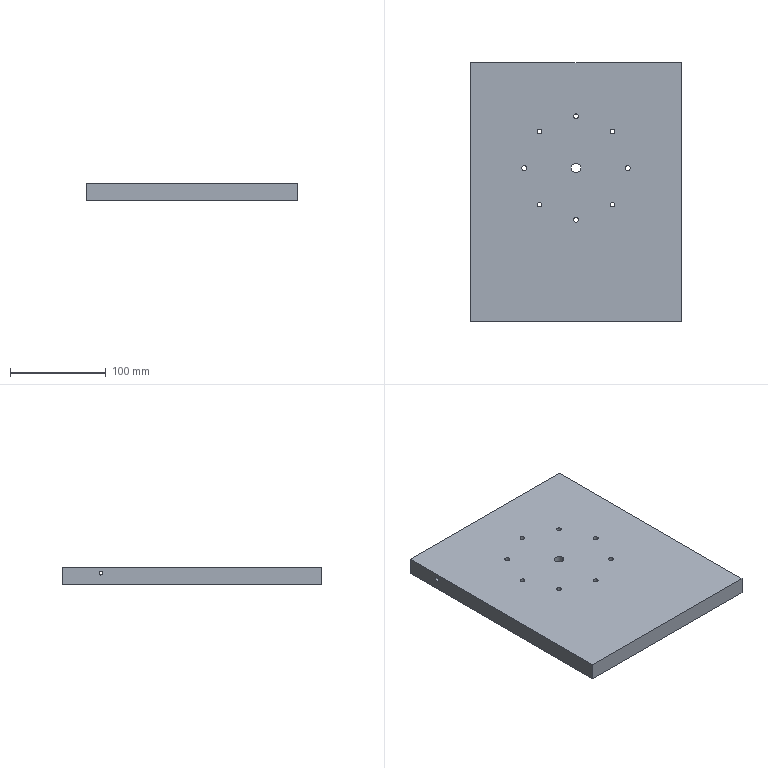Part | SolidWorks | features ICE 5, Extrusion 1 | 1 solid | 26 faces | box 220 x 270 x 18 mm | volume 1062194 mm3 | cylinder 20 | plane 6 | commonest cylinder face diameters 5 x16 4 x2 10 x2
STEP:
#1=CARTESIAN_POINT('',(-110.,100.,14.));
#2=VERTEX_POINT('',#1);
#3=CARTESIAN_POINT('',(-110.,100.,10.));
#4=VERTEX_POINT('',#3);
#5=CARTESIAN_POINT('',(-110.,100.,12.));
#6=DIRECTION('',(1.,0.,0.));
#7=DIRECTION('',(0.,0.,-1.));
#8=AXIS2_PLACEMENT_3D('',#5,#6,#7);
#9=CIRCLE('',#8,2.);
#10=EDGE_CURVE('',#2,#4,#9,.T.);
#11=ORIENTED_EDGE('',*,*,#10,.F.);
#12=CARTESIAN_POINT('',(110.,100.,14.));
#13=VERTEX_POINT('',#12);
#14=CARTESIAN_POINT('',(-110.,100.,14.));
#15=DIRECTION('',(1.,0.,0.));
#16=VECTOR('',#15,1000.);
#17=LINE('',#14,#16);
#18=EDGE_CURVE('',#2,#13,#17,.T.);
#19=ORIENTED_EDGE('',*,*,#18,.T.);
#20=CARTESIAN_POINT('',(110.,100.,10.));
#21=VERTEX_POINT('',#20);
#22=CARTESIAN_POINT('',(110.,100.,12.));
#23=DIRECTION('',(1.,0.,0.));
#24=DIRECTION('',(0.,0.,-1.));
#25=AXIS2_PLACEMENT_3D('',#22,#23,#24);
#26=CIRCLE('',#25,2.);
#27=EDGE_CURVE('',#13,#21,#26,.T.);
#28=ORIENTED_EDGE('',*,*,#27,.T.);
#29=CARTESIAN_POINT('',(-110.,100.,10.));
#30=DIRECTION('',(1.,0.,0.));
#31=VECTOR('',#30,1000.);
#32=LINE('',#29,#31);
#33=EDGE_CURVE('',#4,#21,#32,.T.);
#34=ORIENTED_EDGE('',*,*,#33,.F.);
#35=EDGE_LOOP('',(#11,#19,#28,#34));
#36=FACE_OUTER_BOUND('',#35,.T.);
#37=CARTESIAN_POINT('',(-110.,100.,12.));
#38=DIRECTION('',(1.,0.,0.));
#39=DIRECTION('',(0.,0.,-1.));
#40=AXIS2_PLACEMENT_3D('',#37,#38,#39);
#41=CYLINDRICAL_SURFACE('',#40,2.);
#42=ADVANCED_FACE('',(#36),#41,.F.);
#43=CARTESIAN_POINT('',(-35.684,68.184,18.));
#44=VERTEX_POINT('',#43);
#45=CARTESIAN_POINT('',(-40.684,68.184,18.));
#46=VERTEX_POINT('',#45);
#47=CARTESIAN_POINT('',(-38.184,68.184,18.));
#48=DIRECTION('',(0.,0.,-1.));
#49=DIRECTION('',(-1.,0.,0.));
#50=AXIS2_PLACEMENT_3D('',#47,#48,#49);
#51=CIRCLE('',#50,2.5);
#52=EDGE_CURVE('',#44,#46,#51,.T.);
#53=ORIENTED_EDGE('',*,*,#52,.F.);
#54=CARTESIAN_POINT('',(-35.684,68.184,0.));
#55=VERTEX_POINT('',#54);
#56=CARTESIAN_POINT('',(-35.684,68.184,18.));
#57=DIRECTION('',(0.,0.,-1.));
#58=VECTOR('',#57,1000.);
#59=LINE('',#56,#58);
#60=EDGE_CURVE('',#44,#55,#59,.T.);
#61=ORIENTED_EDGE('',*,*,#60,.T.);
#62=CARTESIAN_POINT('',(-40.684,68.184,0.));
#63=VERTEX_POINT('',#62);
#64=CARTESIAN_POINT('',(-38.184,68.184,0.));
#65=DIRECTION('',(0.,0.,-1.));
#66=DIRECTION('',(-1.,0.,0.));
#67=AXIS2_PLACEMENT_3D('',#64,#65,#66);
#68=CIRCLE('',#67,2.5);
#69=EDGE_CURVE('',#55,#63,#68,.T.);
#70=ORIENTED_EDGE('',*,*,#69,.T.);
#71=CARTESIAN_POINT('',(-40.684,68.184,18.));
#72=DIRECTION('',(0.,0.,-1.));
#73=VECTOR('',#72,1000.);
#74=LINE('',#71,#73);
#75=EDGE_CURVE('',#46,#63,#74,.T.);
#76=ORIENTED_EDGE('',*,*,#75,.F.);
#77=EDGE_LOOP('',(#53,#61,#70,#76));
#78=FACE_OUTER_BOUND('',#77,.T.);
#79=CARTESIAN_POINT('',(-38.184,68.184,18.));
#80=DIRECTION('',(0.,0.,-1.));
#81=DIRECTION('',(-1.,0.,0.));
#82=AXIS2_PLACEMENT_3D('',#79,#80,#81);
#83=CYLINDRICAL_SURFACE('',#82,2.5);
#84=ADVANCED_FACE('',(#78),#83,.F.);
#85=CARTESIAN_POINT('',(-51.5,30.,18.));
#86=VERTEX_POINT('',#85);
#87=CARTESIAN_POINT('',(-56.5,30.,18.));
#88=VERTEX_POINT('',#87);
#89=CARTESIAN_POINT('',(-54.,30.,18.));
#90=DIRECTION('',(0.,0.,-1.));
#91=DIRECTION('',(-1.,0.,0.));
#92=AXIS2_PLACEMENT_3D('',#89,#90,#91);
#93=CIRCLE('',#92,2.5);
#94=EDGE_CURVE('',#86,#88,#93,.T.);
#95=ORIENTED_EDGE('',*,*,#94,.F.);
#96=CARTESIAN_POINT('',(-51.5,30.,0.));
#97=VERTEX_POINT('',#96);
#98=CARTESIAN_POINT('',(-51.5,30.,18.));
#99=DIRECTION('',(0.,0.,-1.));
#100=VECTOR('',#99,1000.);
#101=LINE('',#98,#100);
#102=EDGE_CURVE('',#86,#97,#101,.T.);
#103=ORIENTED_EDGE('',*,*,#102,.T.);
#104=CARTESIAN_POINT('',(-56.5,30.,0.));
#105=VERTEX_POINT('',#104);
#106=CARTESIAN_POINT('',(-54.,30.,0.));
#107=DIRECTION('',(0.,0.,-1.));
#108=DIRECTION('',(-1.,0.,0.));
#109=AXIS2_PLACEMENT_3D('',#106,#107,#108);
#110=CIRCLE('',#109,2.5);
#111=EDGE_CURVE('',#97,#105,#110,.T.);
#112=ORIENTED_EDGE('',*,*,#111,.T.);
#113=CARTESIAN_POINT('',(-56.5,30.,18.));
#114=DIRECTION('',(0.,0.,-1.));
#115=VECTOR('',#114,1000.);
#116=LINE('',#113,#115);
#117=EDGE_CURVE('',#88,#105,#116,.T.);
#118=ORIENTED_EDGE('',*,*,#117,.F.);
#119=EDGE_LOOP('',(#95,#103,#112,#118));
#120=FACE_OUTER_BOUND('',#119,.T.);
#121=CARTESIAN_POINT('',(-54.,30.,18.));
#122=DIRECTION('',(0.,0.,-1.));
#123=DIRECTION('',(-1.,0.,0.));
#124=AXIS2_PLACEMENT_3D('',#121,#122,#123);
#125=CYLINDRICAL_SURFACE('',#124,2.5);
#126=ADVANCED_FACE('',(#120),#125,.F.);
#127=CARTESIAN_POINT('',(-35.684,-8.184,18.));
#128=VERTEX_POINT('',#127);
#129=CARTESIAN_POINT('',(-40.684,-8.184,18.));
#130=VERTEX_POINT('',#129);
#131=CARTESIAN_POINT('',(-38.184,-8.184,18.));
#132=DIRECTION('',(0.,0.,-1.));
#133=DIRECTION('',(-1.,0.,0.));
#134=AXIS2_PLACEMENT_3D('',#131,#132,#133);
#135=CIRCLE('',#134,2.5);
#136=EDGE_CURVE('',#128,#130,#135,.T.);
#137=ORIENTED_EDGE('',*,*,#136,.F.);
#138=CARTESIAN_POINT('',(-35.684,-8.184,0.));
#139=VERTEX_POINT('',#138);
#140=CARTESIAN_POINT('',(-35.684,-8.184,18.));
#141=DIRECTION('',(0.,0.,-1.));
#142=VECTOR('',#141,1000.);
#143=LINE('',#140,#142);
#144=EDGE_CURVE('',#128,#139,#143,.T.);
#145=ORIENTED_EDGE('',*,*,#144,.T.);
#146=CARTESIAN_POINT('',(-40.684,-8.184,0.));
#147=VERTEX_POINT('',#146);
#148=CARTESIAN_POINT('',(-38.184,-8.184,0.));
#149=DIRECTION('',(0.,0.,-1.));
#150=DIRECTION('',(-1.,0.,0.));
#151=AXIS2_PLACEMENT_3D('',#148,#149,#150);
#152=CIRCLE('',#151,2.5);
#153=EDGE_CURVE('',#139,#147,#152,.T.);
#154=ORIENTED_EDGE('',*,*,#153,.T.);
#155=CARTESIAN_POINT('',(-40.684,-8.184,18.));
#156=DIRECTION('',(0.,0.,-1.));
#157=VECTOR('',#156,1000.);
#158=LINE('',#155,#157);
#159=EDGE_CURVE('',#130,#147,#158,.T.);
#160=ORIENTED_EDGE('',*,*,#159,.F.);
#161=EDGE_LOOP('',(#137,#145,#154,#160));
#162=FACE_OUTER_BOUND('',#161,.T.);
#163=CARTESIAN_POINT('',(-38.184,-8.184,18.));
#164=DIRECTION('',(0.,0.,-1.));
#165=DIRECTION('',(-1.,0.,0.));
#166=AXIS2_PLACEMENT_3D('',#163,#164,#165);
#167=CYLINDRICAL_SURFACE('',#166,2.5);
#168=ADVANCED_FACE('',(#162),#167,.F.);
#169=CARTESIAN_POINT('',(2.5,-24.,18.));
#170=VERTEX_POINT('',#169);
#171=CARTESIAN_POINT('',(-2.5,-24.,18.));
#172=VERTEX_POINT('',#171);
#173=CARTESIAN_POINT('',(0.,-24.,18.));
#174=DIRECTION('',(0.,0.,-1.));
#175=DIRECTION('',(-1.,0.,0.));
#176=AXIS2_PLACEMENT_3D('',#173,#174,#175);
#177=CIRCLE('',#176,2.5);
#178=EDGE_CURVE('',#170,#172,#177,.T.);
#179=ORIENTED_EDGE('',*,*,#178,.F.);
#180=CARTESIAN_POINT('',(2.5,-24.,0.));
#181=VERTEX_POINT('',#180);
#182=CARTESIAN_POINT('',(2.5,-24.,18.));
#183=DIRECTION('',(0.,0.,-1.));
#184=VECTOR('',#183,1000.);
#185=LINE('',#182,#184);
#186=EDGE_CURVE('',#170,#181,#185,.T.);
#187=ORIENTED_EDGE('',*,*,#186,.T.);
#188=CARTESIAN_POINT('',(-2.5,-24.,0.));
#189=VERTEX_POINT('',#188);
#190=CARTESIAN_POINT('',(0.,-24.,0.));
#191=DIRECTION('',(0.,0.,-1.));
#192=DIRECTION('',(-1.,0.,0.));
#193=AXIS2_PLACEMENT_3D('',#190,#191,#192);
#194=CIRCLE('',#193,2.5);
#195=EDGE_CURVE('',#181,#189,#194,.T.);
#196=ORIENTED_EDGE('',*,*,#195,.T.);
#197=CARTESIAN_POINT('',(-2.5,-24.,18.));
#198=DIRECTION('',(0.,0.,-1.));
#199=VECTOR('',#198,1000.);
#200=LINE('',#197,#199);
#201=EDGE_CURVE('',#172,#189,#200,.T.);
#202=ORIENTED_EDGE('',*,*,#201,.F.);
#203=EDGE_LOOP('',(#179,#187,#196,#202));
#204=FACE_OUTER_BOUND('',#203,.T.);
#205=CARTESIAN_POINT('',(0.,-24.,18.));
#206=DIRECTION('',(0.,0.,-1.));
#207=DIRECTION('',(-1.,0.,0.));
#208=AXIS2_PLACEMENT_3D('',#205,#206,#207);
#209=CYLINDRICAL_SURFACE('',#208,2.5);
#210=ADVANCED_FACE('',(#204),#209,.F.);
#211=CARTESIAN_POINT('',(40.684,-8.184,18.));
#212=VERTEX_POINT('',#211);
#213=CARTESIAN_POINT('',(35.684,-8.184,18.));
#214=VERTEX_POINT('',#213);
#215=CARTESIAN_POINT('',(38.184,-8.184,18.));
#216=DIRECTION('',(0.,0.,-1.));
#217=DIRECTION('',(-1.,0.,0.));
#218=AXIS2_PLACEMENT_3D('',#215,#216,#217);
#219=CIRCLE('',#218,2.5);
#220=EDGE_CURVE('',#212,#214,#219,.T.);
#221=ORIENTED_EDGE('',*,*,#220,.F.);
#222=CARTESIAN_POINT('',(40.684,-8.184,0.));
#223=VERTEX_POINT('',#222);
#224=CARTESIAN_POINT('',(40.684,-8.184,18.));
#225=DIRECTION('',(0.,0.,-1.));
#226=VECTOR('',#225,1000.);
#227=LINE('',#224,#226);
#228=EDGE_CURVE('',#212,#223,#227,.T.);
#229=ORIENTED_EDGE('',*,*,#228,.T.);
#230=CARTESIAN_POINT('',(35.684,-8.184,0.));
#231=VERTEX_POINT('',#230);
#232=CARTESIAN_POINT('',(38.184,-8.184,0.));
#233=DIRECTION('',(0.,0.,-1.));
#234=DIRECTION('',(-1.,0.,0.));
#235=AXIS2_PLACEMENT_3D('',#232,#233,#234);
#236=CIRCLE('',#235,2.5);
#237=EDGE_CURVE('',#223,#231,#236,.T.);
#238=ORIENTED_EDGE('',*,*,#237,.T.);
#239=CARTESIAN_POINT('',(35.684,-8.184,18.));
#240=DIRECTION('',(0.,0.,-1.));
#241=VECTOR('',#240,1000.);
#242=LINE('',#239,#241);
#243=EDGE_CURVE('',#214,#231,#242,.T.);
#244=ORIENTED_EDGE('',*,*,#243,.F.);
#245=EDGE_LOOP('',(#221,#229,#238,#244));
#246=FACE_OUTER_BOUND('',#245,.T.);
#247=CARTESIAN_POINT('',(38.184,-8.184,18.));
#248=DIRECTION('',(0.,0.,-1.));
#249=DIRECTION('',(-1.,0.,0.));
#250=AXIS2_PLACEMENT_3D('',#247,#248,#249);
#251=CYLINDRICAL_SURFACE('',#250,2.5);
#252=ADVANCED_FACE('',(#246),#251,.F.);
#253=CARTESIAN_POINT('',(56.5,30.,18.));
#254=VERTEX_POINT('',#253);
#255=CARTESIAN_POINT('',(51.5,30.,18.));
#256=VERTEX_POINT('',#255);
#257=CARTESIAN_POINT('',(54.,30.,18.));
#258=DIRECTION('',(0.,0.,-1.));
#259=DIRECTION('',(-1.,0.,0.));
#260=AXIS2_PLACEMENT_3D('',#257,#258,#259);
#261=CIRCLE('',#260,2.5);
#262=EDGE_CURVE('',#254,#256,#261,.T.);
#263=ORIENTED_EDGE('',*,*,#262,.F.);
#264=CARTESIAN_POINT('',(56.5,30.,0.));
#265=VERTEX_POINT('',#264);
#266=CARTESIAN_POINT('',(56.5,30.,18.));
#267=DIRECTION('',(0.,0.,-1.));
#268=VECTOR('',#267,1000.);
#269=LINE('',#266,#268);
#270=EDGE_CURVE('',#254,#265,#269,.T.);
#271=ORIENTED_EDGE('',*,*,#270,.T.);
#272=CARTESIAN_POINT('',(51.5,30.,0.));
#273=VERTEX_POINT('',#272);
#274=CARTESIAN_POINT('',(54.,30.,0.));
#275=DIRECTION('',(0.,0.,-1.));
#276=DIRECTION('',(-1.,0.,0.));
#277=AXIS2_PLACEMENT_3D('',#274,#275,#276);
#278=CIRCLE('',#277,2.5);
#279=EDGE_CURVE('',#265,#273,#278,.T.);
#280=ORIENTED_EDGE('',*,*,#279,.T.);
#281=CARTESIAN_POINT('',(51.5,30.,18.));
#282=DIRECTION('',(0.,0.,-1.));
#283=VECTOR('',#282,1000.);
#284=LINE('',#281,#283);
#285=EDGE_CURVE('',#256,#273,#284,.T.);
#286=ORIENTED_EDGE('',*,*,#285,.F.);
#287=EDGE_LOOP('',(#263,#271,#280,#286));
#288=FACE_OUTER_BOUND('',#287,.T.);
#289=CARTESIAN_POINT('',(54.,30.,18.));
#290=DIRECTION('',(0.,0.,-1.));
#291=DIRECTION('',(-1.,0.,0.));
#292=AXIS2_PLACEMENT_3D('',#289,#290,#291);
#293=CYLINDRICAL_SURFACE('',#292,2.5);
#294=ADVANCED_FACE('',(#288),#293,.F.);
#295=CARTESIAN_POINT('',(2.5,84.,18.));
#296=VERTEX_POINT('',#295);
#297=CARTESIAN_POINT('',(-2.5,84.,18.));
#298=VERTEX_POINT('',#297);
#299=CARTESIAN_POINT('',(0.,84.,18.));
#300=DIRECTION('',(0.,0.,-1.));
#301=DIRECTION('',(-1.,0.,0.));
#302=AXIS2_PLACEMENT_3D('',#299,#300,#301);
#303=CIRCLE('',#302,2.5);
#304=EDGE_CURVE('',#296,#298,#303,.T.);
#305=ORIENTED_EDGE('',*,*,#304,.F.);
#306=CARTESIAN_POINT('',(2.5,84.,0.));
#307=VERTEX_POINT('',#306);
#308=CARTESIAN_POINT('',(2.5,84.,18.));
#309=DIRECTION('',(0.,0.,-1.));
#310=VECTOR('',#309,1000.);
#311=LINE('',#308,#310);
#312=EDGE_CURVE('',#296,#307,#311,.T.);
#313=ORIENTED_EDGE('',*,*,#312,.T.);
#314=CARTESIAN_POINT('',(-2.5,84.,0.));
#315=VERTEX_POINT('',#314);
#316=CARTESIAN_POINT('',(0.,84.,0.));
#317=DIRECTION('',(0.,0.,-1.));
#318=DIRECTION('',(-1.,0.,0.));
#319=AXIS2_PLACEMENT_3D('',#316,#317,#318);
#320=CIRCLE('',#319,2.5);
#321=EDGE_CURVE('',#307,#315,#320,.T.);
#322=ORIENTED_EDGE('',*,*,#321,.T.);
#323=CARTESIAN_POINT('',(-2.5,84.,18.));
#324=DIRECTION('',(0.,0.,-1.));
#325=VECTOR('',#324,1000.);
#326=LINE('',#323,#325);
#327=EDGE_CURVE('',#298,#315,#326,.T.);
#328=ORIENTED_EDGE('',*,*,#327,.F.);
#329=EDGE_LOOP('',(#305,#313,#322,#328));
#330=FACE_OUTER_BOUND('',#329,.T.);
#331=CARTESIAN_POINT('',(0.,84.,18.));
#332=DIRECTION('',(0.,0.,-1.));
#333=DIRECTION('',(-1.,0.,0.));
#334=AXIS2_PLACEMENT_3D('',#331,#332,#333);
#335=CYLINDRICAL_SURFACE('',#334,2.5);
#336=ADVANCED_FACE('',(#330),#335,.F.);
#337=CARTESIAN_POINT('',(40.684,68.184,18.));
#338=VERTEX_POINT('',#337);
#339=CARTESIAN_POINT('',(35.684,68.184,18.));
#340=VERTEX_POINT('',#339);
#341=CARTESIAN_POINT('',(38.184,68.184,18.));
#342=DIRECTION('',(0.,0.,-1.));
#343=DIRECTION('',(-1.,0.,0.));
#344=AXIS2_PLACEMENT_3D('',#341,#342,#343);
#345=CIRCLE('',#344,2.5);
#346=EDGE_CURVE('',#338,#340,#345,.T.);
#347=ORIENTED_EDGE('',*,*,#346,.F.);
#348=CARTESIAN_POINT('',(40.684,68.184,0.));
#349=VERTEX_POINT('',#348);
#350=CARTESIAN_POINT('',(40.684,68.184,18.));
#351=DIRECTION('',(0.,0.,-1.));
#352=VECTOR('',#351,1000.);
#353=LINE('',#350,#352);
#354=EDGE_CURVE('',#338,#349,#353,.T.);
#355=ORIENTED_EDGE('',*,*,#354,.T.);
#356=CARTESIAN_POINT('',(35.684,68.184,0.));
#357=VERTEX_POINT('',#356);
#358=CARTESIAN_POINT('',(38.184,68.184,0.));
#359=DIRECTION('',(0.,0.,-1.));
#360=DIRECTION('',(-1.,0.,0.));
#361=AXIS2_PLACEMENT_3D('',#358,#359,#360);
#362=CIRCLE('',#361,2.5);
#363=EDGE_CURVE('',#349,#357,#362,.T.);
#364=ORIENTED_EDGE('',*,*,#363,.T.);
#365=CARTESIAN_POINT('',(35.684,68.184,18.));
#366=DIRECTION('',(0.,0.,-1.));
#367=VECTOR('',#366,1000.);
#368=LINE('',#365,#367);
#369=EDGE_CURVE('',#340,#357,#368,.T.);
#370=ORIENTED_EDGE('',*,*,#369,.F.);
#371=EDGE_LOOP('',(#347,#355,#364,#370));
#372=FACE_OUTER_BOUND('',#371,.T.);
#373=CARTESIAN_POINT('',(38.184,68.184,18.));
#374=DIRECTION('',(0.,0.,-1.));
#375=DIRECTION('',(-1.,0.,0.));
#376=AXIS2_PLACEMENT_3D('',#373,#374,#375);
#377=CYLINDRICAL_SURFACE('',#376,2.5);
#378=ADVANCED_FACE('',(#372),#377,.F.);
#379=CARTESIAN_POINT('',(-5.,30.,18.));
#380=VERTEX_POINT('',#379);
#381=CARTESIAN_POINT('',(5.,30.,18.));
#382=VERTEX_POINT('',#381);
#383=CARTESIAN_POINT('',(0.,30.,18.));
#384=DIRECTION('',(0.,0.,1.));
#385=DIRECTION('',(1.,0.,0.));
#386=AXIS2_PLACEMENT_3D('',#383,#384,#385);
#387=CIRCLE('',#386,5.);
#388=EDGE_CURVE('',#380,#382,#387,.T.);
#389=ORIENTED_EDGE('',*,*,#388,.T.);
#390=CARTESIAN_POINT('',(5.,30.,0.));
#391=VERTEX_POINT('',#390);
#392=CARTESIAN_POINT('',(5.,30.,18.));
#393=DIRECTION('',(0.,0.,-1.));
#394=VECTOR('',#393,1000.);
#395=LINE('',#392,#394);
#396=EDGE_CURVE('',#382,#391,#395,.T.);
#397=ORIENTED_EDGE('',*,*,#396,.T.);
#398=CARTESIAN_POINT('',(-5.,30.,0.));
#399=VERTEX_POINT('',#398);
#400=CARTESIAN_POINT('',(0.,30.,0.));
#401=DIRECTION('',(0.,0.,1.));
#402=DIRECTION('',(1.,0.,0.));
#403=AXIS2_PLACEMENT_3D('',#400,#401,#402);
#404=CIRCLE('',#403,5.);
#405=EDGE_CURVE('',#399,#391,#404,.T.);
#406=ORIENTED_EDGE('',*,*,#405,.F.);
#407=CARTESIAN_POINT('',(-5.,30.,18.));
#408=DIRECTION('',(0.,0.,-1.));
#409=VECTOR('',#408,1000.);
#410=LINE('',#407,#409);
#411=EDGE_CURVE('',#380,#399,#410,.T.);
#412=ORIENTED_EDGE('',*,*,#411,.F.);
#413=EDGE_LOOP('',(#389,#397,#406,#412));
#414=FACE_OUTER_BOUND('',#413,.T.);
#415=CARTESIAN_POINT('',(0.,30.,18.));
#416=DIRECTION('',(0.,0.,-1.));
#417=DIRECTION('',(-1.,0.,0.));
#418=AXIS2_PLACEMENT_3D('',#415,#416,#417);
#419=CYLINDRICAL_SURFACE('',#418,5.);
#420=ADVANCED_FACE('',(#414),#419,.F.);
#421=CARTESIAN_POINT('',(110.,100.,12.));
#422=DIRECTION('',(1.,0.,0.));
#423=DIRECTION('',(0.,0.,-1.));
#424=AXIS2_PLACEMENT_3D('',#421,#422,#423);
#425=CIRCLE('',#424,2.);
#426=EDGE_CURVE('',#21,#13,#425,.T.);
#427=ORIENTED_EDGE('',*,*,#426,.F.);
#428=ORIENTED_EDGE('',*,*,#27,.F.);
#429=EDGE_LOOP('',(#427,#428));
#430=FACE_BOUND('',#429,.T.);
#431=CARTESIAN_POINT('',(110.,-130.,18.));
#432=VERTEX_POINT('',#431);
#433=CARTESIAN_POINT('',(110.,140.,18.));
#434=VERTEX_POINT('',#433);
#435=CARTESIAN_POINT('',(110.,-140.,18.));
#436=DIRECTION('',(0.,1.,0.));
#437=VECTOR('',#436,1000.);
#438=LINE('',#435,#437);
#439=EDGE_CURVE('',#432,#434,#438,.T.);
#440=ORIENTED_EDGE('',*,*,#439,.F.);
#441=CARTESIAN_POINT('',(110.,-130.,0.));
#442=VERTEX_POINT('',#441);
#443=CARTESIAN_POINT('',(110.,-130.,0.));
#444=DIRECTION('',(0.,0.,1.));
#445=VECTOR('',#444,1000.);
#446=LINE('',#443,#445);
#447=EDGE_CURVE('',#442,#432,#446,.T.);
#448=ORIENTED_EDGE('',*,*,#447,.F.);
#449=CARTESIAN_POINT('',(110.,140.,0.));
#450=VERTEX_POINT('',#449);
#451=CARTESIAN_POINT('',(110.,-140.,0.));
#452=DIRECTION('',(0.,1.,0.));
#453=VECTOR('',#452,1000.);
#454=LINE('',#451,#453);
#455=EDGE_CURVE('',#442,#450,#454,.T.);
#456=ORIENTED_EDGE('',*,*,#455,.T.);
#457=CARTESIAN_POINT('',(110.,140.,18.));
#458=DIRECTION('',(0.,0.,-1.));
#459=VECTOR('',#458,1000.);
#460=LINE('',#457,#459);
#461=EDGE_CURVE('',#434,#450,#460,.T.);
#462=ORIENTED_EDGE('',*,*,#461,.F.);
#463=EDGE_LOOP('',(#440,#448,#456,#462));
#464=FACE_OUTER_BOUND('',#463,.T.);
#465=CARTESIAN_POINT('',(110.,-140.,18.));
#466=DIRECTION('',(-1.,0.,0.));
#467=DIRECTION('',(0.,0.,1.));
#468=AXIS2_PLACEMENT_3D('',#465,#466,#467);
#469=PLANE('',#468);
#470=ADVANCED_FACE('',(#430,#464),#469,.F.);
#471=CARTESIAN_POINT('',(-110.,100.,12.));
#472=DIRECTION('',(1.,0.,0.));
#473=DIRECTION('',(0.,0.,-1.));
#474=AXIS2_PLACEMENT_3D('',#471,#472,#473);
#475=CIRCLE('',#474,2.);
#476=EDGE_CURVE('',#4,#2,#475,.T.);
#477=ORIENTED_EDGE('',*,*,#476,.T.);
#478=ORIENTED_EDGE('',*,*,#10,.T.);
#479=EDGE_LOOP('',(#477,#478));
#480=FACE_BOUND('',#479,.T.);
#481=CARTESIAN_POINT('',(-110.,140.,0.));
#482=VERTEX_POINT('',#481);
#483=CARTESIAN_POINT('',(-110.,-130.,0.));
#484=VERTEX_POINT('',#483);
#485=CARTESIAN_POINT('',(-110.,-140.,0.));
#486=DIRECTION('',(0.,-1.,0.));
#487=VECTOR('',#486,1000.);
#488=LINE('',#485,#487);
#489=EDGE_CURVE('',#482,#484,#488,.T.);
#490=ORIENTED_EDGE('',*,*,#489,.T.);
#491=CARTESIAN_POINT('',(-110.,-130.,18.));
#492=VERTEX_POINT('',#491);
#493=CARTESIAN_POINT('',(-110.,-130.,0.));
#494=DIRECTION('',(0.,0.,1.));
#495=VECTOR('',#494,1000.);
#496=LINE('',#493,#495);
#497=EDGE_CURVE('',#484,#492,#496,.T.);
#498=ORIENTED_EDGE('',*,*,#497,.T.);
#499=CARTESIAN_POINT('',(-110.,140.,18.));
#500=VERTEX_POINT('',#499);
#501=CARTESIAN_POINT('',(-110.,-140.,18.));
#502=DIRECTION('',(0.,-1.,0.));
#503=VECTOR('',#502,1000.);
#504=LINE('',#501,#503);
#505=EDGE_CURVE('',#500,#492,#504,.T.);
#506=ORIENTED_EDGE('',*,*,#505,.F.);
#507=CARTESIAN_POINT('',(-110.,140.,18.));
#508=DIRECTION('',(0.,0.,-1.));
#509=VECTOR('',#508,1000.);
#510=LINE('',#507,#509);
#511=EDGE_CURVE('',#500,#482,#510,.T.);
#512=ORIENTED_EDGE('',*,*,#511,.T.);
#513=EDGE_LOOP('',(#490,#498,#506,#512));
#514=FACE_OUTER_BOUND('',#513,.T.);
#515=CARTESIAN_POINT('',(-110.,-140.,18.));
#516=DIRECTION('',(1.,0.,0.));
#517=DIRECTION('',(0.,0.,-1.));
#518=AXIS2_PLACEMENT_3D('',#515,#516,#517);
#519=PLANE('',#518);
#520=ADVANCED_FACE('',(#480,#514),#519,.F.);
#521=CARTESIAN_POINT('',(-38.184,68.184,18.));
#522=DIRECTION('',(0.,0.,-1.));
#523=DIRECTION('',(-1.,0.,0.));
#524=AXIS2_PLACEMENT_3D('',#521,#522,#523);
#525=CIRCLE('',#524,2.5);
#526=EDGE_CURVE('',#46,#44,#525,.T.);
#527=ORIENTED_EDGE('',*,*,#526,.T.);
#528=ORIENTED_EDGE('',*,*,#52,.T.);
#529=EDGE_LOOP('',(#527,#528));
#530=FACE_BOUND('',#529,.T.);
#531=CARTESIAN_POINT('',(-54.,30.,18.));
#532=DIRECTION('',(0.,0.,-1.));
#533=DIRECTION('',(-1.,0.,0.));
#534=AXIS2_PLACEMENT_3D('',#531,#532,#533);
#535=CIRCLE('',#534,2.5);
#536=EDGE_CURVE('',#88,#86,#535,.T.);
#537=ORIENTED_EDGE('',*,*,#536,.T.);
#538=ORIENTED_EDGE('',*,*,#94,.T.);
#539=EDGE_LOOP('',(#537,#538));
#540=FACE_BOUND('',#539,.T.);
#541=CARTESIAN_POINT('',(-38.184,-8.184,18.));
#542=DIRECTION('',(0.,0.,-1.));
#543=DIRECTION('',(-1.,0.,0.));
#544=AXIS2_PLACEMENT_3D('',#541,#542,#543);
#545=CIRCLE('',#544,2.5);
#546=EDGE_CURVE('',#130,#128,#545,.T.);
#547=ORIENTED_EDGE('',*,*,#546,.T.);
#548=ORIENTED_EDGE('',*,*,#136,.T.);
#549=EDGE_LOOP('',(#547,#548));
#550=FACE_BOUND('',#549,.T.);
#551=CARTESIAN_POINT('',(0.,-24.,18.));
#552=DIRECTION('',(0.,0.,-1.));
#553=DIRECTION('',(-1.,0.,0.));
#554=AXIS2_PLACEMENT_3D('',#551,#552,#553);
#555=CIRCLE('',#554,2.5);
#556=EDGE_CURVE('',#172,#170,#555,.T.);
#557=ORIENTED_EDGE('',*,*,#556,.T.);
#558=ORIENTED_EDGE('',*,*,#178,.T.);
#559=EDGE_LOOP('',(#557,#558));
#560=FACE_BOUND('',#559,.T.);
#561=CARTESIAN_POINT('',(38.184,-8.184,18.));
#562=DIRECTION('',(0.,0.,-1.));
#563=DIRECTION('',(-1.,0.,0.));
#564=AXIS2_PLACEMENT_3D('',#561,#562,#563);
#565=CIRCLE('',#564,2.5);
#566=EDGE_CURVE('',#214,#212,#565,.T.);
#567=ORIENTED_EDGE('',*,*,#566,.T.);
#568=ORIENTED_EDGE('',*,*,#220,.T.);
#569=EDGE_LOOP('',(#567,#568));
#570=FACE_BOUND('',#569,.T.);
#571=CARTESIAN_POINT('',(54.,30.,18.));
#572=DIRECTION('',(0.,0.,-1.));
#573=DIRECTION('',(-1.,0.,0.));
#574=AXIS2_PLACEMENT_3D('',#571,#572,#573);
#575=CIRCLE('',#574,2.5);
#576=EDGE_CURVE('',#256,#254,#575,.T.);
#577=ORIENTED_EDGE('',*,*,#576,.T.);
#578=ORIENTED_EDGE('',*,*,#262,.T.);
#579=EDGE_LOOP('',(#577,#578));
#580=FACE_BOUND('',#579,.T.);
#581=CARTESIAN_POINT('',(0.,84.,18.));
#582=DIRECTION('',(0.,0.,-1.));
#583=DIRECTION('',(-1.,0.,0.));
#584=AXIS2_PLACEMENT_3D('',#581,#582,#583);
#585=CIRCLE('',#584,2.5);
#586=EDGE_CURVE('',#298,#296,#585,.T.);
#587=ORIENTED_EDGE('',*,*,#586,.T.);
#588=ORIENTED_EDGE('',*,*,#304,.T.);
#589=EDGE_LOOP('',(#587,#588));
#590=FACE_BOUND('',#589,.T.);
#591=CARTESIAN_POINT('',(38.184,68.184,18.));
#592=DIRECTION('',(0.,0.,-1.));
#593=DIRECTION('',(-1.,0.,0.));
#594=AXIS2_PLACEMENT_3D('',#591,#592,#593);
#595=CIRCLE('',#594,2.5);
#596=EDGE_CURVE('',#340,#338,#595,.T.);
#597=ORIENTED_EDGE('',*,*,#596,.T.);
#598=ORIENTED_EDGE('',*,*,#346,.T.);
#599=EDGE_LOOP('',(#597,#598));
#600=FACE_BOUND('',#599,.T.);
#601=ORIENTED_EDGE('',*,*,#388,.F.);
#602=CARTESIAN_POINT('',(0.,30.,18.));
#603=DIRECTION('',(0.,0.,1.));
#604=DIRECTION('',(1.,0.,0.));
#605=AXIS2_PLACEMENT_3D('',#602,#603,#604);
#606=CIRCLE('',#605,5.);
#607=EDGE_CURVE('',#382,#380,#606,.T.);
#608=ORIENTED_EDGE('',*,*,#607,.F.);
#609=EDGE_LOOP('',(#601,#608));
#610=FACE_BOUND('',#609,.T.);
#611=ORIENTED_EDGE('',*,*,#505,.T.);
#612=CARTESIAN_POINT('',(110.,-130.,18.));
#613=DIRECTION('',(-1.,0.,0.));
#614=VECTOR('',#613,1000.);
#615=LINE('',#612,#614);
#616=EDGE_CURVE('',#432,#492,#615,.T.);
#617=ORIENTED_EDGE('',*,*,#616,.F.);
#618=ORIENTED_EDGE('',*,*,#439,.T.);
#619=CARTESIAN_POINT('',(-110.,140.,18.));
#620=DIRECTION('',(-1.,0.,0.));
#621=VECTOR('',#620,1000.);
#622=LINE('',#619,#621);
#623=EDGE_CURVE('',#434,#500,#622,.T.);
#624=ORIENTED_EDGE('',*,*,#623,.T.);
#625=EDGE_LOOP('',(#611,#617,#618,#624));
#626=FACE_OUTER_BOUND('',#625,.T.);
#627=CARTESIAN_POINT('',(0.,0.,18.));
#628=DIRECTION('',(0.,0.,-1.));
#629=DIRECTION('',(-1.,0.,0.));
#630=AXIS2_PLACEMENT_3D('',#627,#628,#629);
#631=PLANE('',#630);
#632=ADVANCED_FACE('',(#530,#540,#550,#560,#570,#580,#590,#600,#610,#626),#631,.F.);
#633=CARTESIAN_POINT('',(-38.184,68.184,0.));
#634=DIRECTION('',(0.,0.,-1.));
#635=DIRECTION('',(-1.,0.,0.));
#636=AXIS2_PLACEMENT_3D('',#633,#634,#635);
#637=CIRCLE('',#636,2.5);
#638=EDGE_CURVE('',#63,#55,#637,.T.);
#639=ORIENTED_EDGE('',*,*,#638,.F.);
#640=ORIENTED_EDGE('',*,*,#69,.F.);
#641=EDGE_LOOP('',(#639,#640));
#642=FACE_BOUND('',#641,.T.);
#643=CARTESIAN_POINT('',(-54.,30.,0.));
#644=DIRECTION('',(0.,0.,-1.));
#645=DIRECTION('',(-1.,0.,0.));
#646=AXIS2_PLACEMENT_3D('',#643,#644,#645);
#647=CIRCLE('',#646,2.5);
#648=EDGE_CURVE('',#105,#97,#647,.T.);
#649=ORIENTED_EDGE('',*,*,#648,.F.);
#650=ORIENTED_EDGE('',*,*,#111,.F.);
#651=EDGE_LOOP('',(#649,#650));
#652=FACE_BOUND('',#651,.T.);
#653=CARTESIAN_POINT('',(-38.184,-8.184,0.));
#654=DIRECTION('',(0.,0.,-1.));
#655=DIRECTION('',(-1.,0.,0.));
#656=AXIS2_PLACEMENT_3D('',#653,#654,#655);
#657=CIRCLE('',#656,2.5);
#658=EDGE_CURVE('',#147,#139,#657,.T.);
#659=ORIENTED_EDGE('',*,*,#658,.F.);
#660=ORIENTED_EDGE('',*,*,#153,.F.);
#661=EDGE_LOOP('',(#659,#660));
#662=FACE_BOUND('',#661,.T.);
#663=CARTESIAN_POINT('',(0.,-24.,0.));
#664=DIRECTION('',(0.,0.,-1.));
#665=DIRECTION('',(-1.,0.,0.));
#666=AXIS2_PLACEMENT_3D('',#663,#664,#665);
#667=CIRCLE('',#666,2.5);
#668=EDGE_CURVE('',#189,#181,#667,.T.);
#669=ORIENTED_EDGE('',*,*,#668,.F.);
#670=ORIENTED_EDGE('',*,*,#195,.F.);
#671=EDGE_LOOP('',(#669,#670));
#672=FACE_BOUND('',#671,.T.);
#673=CARTESIAN_POINT('',(38.184,-8.184,0.));
#674=DIRECTION('',(0.,0.,-1.));
#675=DIRECTION('',(-1.,0.,0.));
#676=AXIS2_PLACEMENT_3D('',#673,#674,#675);
#677=CIRCLE('',#676,2.5);
#678=EDGE_CURVE('',#231,#223,#677,.T.);
#679=ORIENTED_EDGE('',*,*,#678,.F.);
#680=ORIENTED_EDGE('',*,*,#237,.F.);
#681=EDGE_LOOP('',(#679,#680));
#682=FACE_BOUND('',#681,.T.);
#683=CARTESIAN_POINT('',(54.,30.,0.));
#684=DIRECTION('',(0.,0.,-1.));
#685=DIRECTION('',(-1.,0.,0.));
#686=AXIS2_PLACEMENT_3D('',#683,#684,#685);
#687=CIRCLE('',#686,2.5);
#688=EDGE_CURVE('',#273,#265,#687,.T.);
#689=ORIENTED_EDGE('',*,*,#688,.F.);
#690=ORIENTED_EDGE('',*,*,#279,.F.);
#691=EDGE_LOOP('',(#689,#690));
#692=FACE_BOUND('',#691,.T.);
#693=CARTESIAN_POINT('',(0.,84.,0.));
#694=DIRECTION('',(0.,0.,-1.));
#695=DIRECTION('',(-1.,0.,0.));
#696=AXIS2_PLACEMENT_3D('',#693,#694,#695);
#697=CIRCLE('',#696,2.5);
#698=EDGE_CURVE('',#315,#307,#697,.T.);
#699=ORIENTED_EDGE('',*,*,#698,.F.);
#700=ORIENTED_EDGE('',*,*,#321,.F.);
#701=EDGE_LOOP('',(#699,#700));
#702=FACE_BOUND('',#701,.T.);
#703=CARTESIAN_POINT('',(38.184,68.184,0.));
#704=DIRECTION('',(0.,0.,-1.));
#705=DIRECTION('',(-1.,0.,0.));
#706=AXIS2_PLACEMENT_3D('',#703,#704,#705);
#707=CIRCLE('',#706,2.5);
#708=EDGE_CURVE('',#357,#349,#707,.T.);
#709=ORIENTED_EDGE('',*,*,#708,.F.);
#710=ORIENTED_EDGE('',*,*,#363,.F.);
#711=EDGE_LOOP('',(#709,#710));
#712=FACE_BOUND('',#711,.T.);
#713=ORIENTED_EDGE('',*,*,#405,.T.);
#714=CARTESIAN_POINT('',(0.,30.,0.));
#715=DIRECTION('',(0.,0.,1.));
#716=DIRECTION('',(1.,0.,0.));
#717=AXIS2_PLACEMENT_3D('',#714,#715,#716);
#718=CIRCLE('',#717,5.);
#719=EDGE_CURVE('',#391,#399,#718,.T.);
#720=ORIENTED_EDGE('',*,*,#719,.T.);
#721=EDGE_LOOP('',(#713,#720));
#722=FACE_BOUND('',#721,.T.);
#723=ORIENTED_EDGE('',*,*,#455,.F.);
#724=CARTESIAN_POINT('',(110.,-130.,0.));
#725=DIRECTION('',(-1.,0.,0.));
#726=VECTOR('',#725,1000.);
#727=LINE('',#724,#726);
#728=EDGE_CURVE('',#442,#484,#727,.T.);
#729=ORIENTED_EDGE('',*,*,#728,.T.);
#730=ORIENTED_EDGE('',*,*,#489,.F.);
#731=CARTESIAN_POINT('',(-110.,140.,0.));
#732=DIRECTION('',(-1.,0.,0.));
#733=VECTOR('',#732,1000.);
#734=LINE('',#731,#733);
#735=EDGE_CURVE('',#450,#482,#734,.T.);
#736=ORIENTED_EDGE('',*,*,#735,.F.);
#737=EDGE_LOOP('',(#723,#729,#730,#736));
#738=FACE_OUTER_BOUND('',#737,.T.);
#739=CARTESIAN_POINT('',(0.,0.,0.));
#740=DIRECTION('',(0.,0.,-1.));
#741=DIRECTION('',(-1.,0.,0.));
#742=AXIS2_PLACEMENT_3D('',#739,#740,#741);
#743=PLANE('',#742);
#744=ADVANCED_FACE('',(#642,#652,#662,#672,#682,#692,#702,#712,#722,#738),#743,.T.);
#745=ORIENTED_EDGE('',*,*,#735,.T.);
#746=ORIENTED_EDGE('',*,*,#511,.F.);
#747=ORIENTED_EDGE('',*,*,#623,.F.);
#748=ORIENTED_EDGE('',*,*,#461,.T.);
#749=EDGE_LOOP('',(#745,#746,#747,#748));
#750=FACE_OUTER_BOUND('',#749,.T.);
#751=CARTESIAN_POINT('',(-110.,140.,18.));
#752=DIRECTION('',(0.,-1.,0.));
#753=DIRECTION('',(0.,0.,-1.));
#754=AXIS2_PLACEMENT_3D('',#751,#752,#753);
#755=PLANE('',#754);
#756=ADVANCED_FACE('',(#750),#755,.F.);
#757=ORIENTED_EDGE('',*,*,#396,.F.);
#758=ORIENTED_EDGE('',*,*,#607,.T.);
#759=ORIENTED_EDGE('',*,*,#411,.T.);
#760=ORIENTED_EDGE('',*,*,#719,.F.);
#761=EDGE_LOOP('',(#757,#758,#759,#760));
#762=FACE_OUTER_BOUND('',#761,.T.);
#763=CARTESIAN_POINT('',(0.,30.,18.));
#764=DIRECTION('',(0.,0.,-1.));
#765=DIRECTION('',(-1.,0.,0.));
#766=AXIS2_PLACEMENT_3D('',#763,#764,#765);
#767=CYLINDRICAL_SURFACE('',#766,5.);
#768=ADVANCED_FACE('',(#762),#767,.F.);
#769=ORIENTED_EDGE('',*,*,#354,.F.);
#770=ORIENTED_EDGE('',*,*,#596,.F.);
#771=ORIENTED_EDGE('',*,*,#369,.T.);
#772=ORIENTED_EDGE('',*,*,#708,.T.);
#773=EDGE_LOOP('',(#769,#770,#771,#772));
#774=FACE_OUTER_BOUND('',#773,.T.);
#775=CARTESIAN_POINT('',(38.184,68.184,18.));
#776=DIRECTION('',(0.,0.,-1.));
#777=DIRECTION('',(-1.,0.,0.));
#778=AXIS2_PLACEMENT_3D('',#775,#776,#777);
#779=CYLINDRICAL_SURFACE('',#778,2.5);
#780=ADVANCED_FACE('',(#774),#779,.F.);
#781=ORIENTED_EDGE('',*,*,#312,.F.);
#782=ORIENTED_EDGE('',*,*,#586,.F.);
#783=ORIENTED_EDGE('',*,*,#327,.T.);
#784=ORIENTED_EDGE('',*,*,#698,.T.);
#785=EDGE_LOOP('',(#781,#782,#783,#784));
#786=FACE_OUTER_BOUND('',#785,.T.);
#787=CARTESIAN_POINT('',(0.,84.,18.));
#788=DIRECTION('',(0.,0.,-1.));
#789=DIRECTION('',(-1.,0.,0.));
#790=AXIS2_PLACEMENT_3D('',#787,#788,#789);
#791=CYLINDRICAL_SURFACE('',#790,2.5);
#792=ADVANCED_FACE('',(#786),#791,.F.);
#793=ORIENTED_EDGE('',*,*,#270,.F.);
#794=ORIENTED_EDGE('',*,*,#576,.F.);
#795=ORIENTED_EDGE('',*,*,#285,.T.);
#796=ORIENTED_EDGE('',*,*,#688,.T.);
#797=EDGE_LOOP('',(#793,#794,#795,#796));
#798=FACE_OUTER_BOUND('',#797,.T.);
#799=CARTESIAN_POINT('',(54.,30.,18.));
#800=DIRECTION('',(0.,0.,-1.));
#801=DIRECTION('',(-1.,0.,0.));
#802=AXIS2_PLACEMENT_3D('',#799,#800,#801);
#803=CYLINDRICAL_SURFACE('',#802,2.5);
#804=ADVANCED_FACE('',(#798),#803,.F.);
#805=ORIENTED_EDGE('',*,*,#228,.F.);
#806=ORIENTED_EDGE('',*,*,#566,.F.);
#807=ORIENTED_EDGE('',*,*,#243,.T.);
#808=ORIENTED_EDGE('',*,*,#678,.T.);
#809=EDGE_LOOP('',(#805,#806,#807,#808));
#810=FACE_OUTER_BOUND('',#809,.T.);
#811=CARTESIAN_POINT('',(38.184,-8.184,18.));
#812=DIRECTION('',(0.,0.,-1.));
#813=DIRECTION('',(-1.,0.,0.));
#814=AXIS2_PLACEMENT_3D('',#811,#812,#813);
#815=CYLINDRICAL_SURFACE('',#814,2.5);
#816=ADVANCED_FACE('',(#810),#815,.F.);
#817=ORIENTED_EDGE('',*,*,#186,.F.);
#818=ORIENTED_EDGE('',*,*,#556,.F.);
#819=ORIENTED_EDGE('',*,*,#201,.T.);
#820=ORIENTED_EDGE('',*,*,#668,.T.);
#821=EDGE_LOOP('',(#817,#818,#819,#820));
#822=FACE_OUTER_BOUND('',#821,.T.);
#823=CARTESIAN_POINT('',(0.,-24.,18.));
#824=DIRECTION('',(0.,0.,-1.));
#825=DIRECTION('',(-1.,0.,0.));
#826=AXIS2_PLACEMENT_3D('',#823,#824,#825);
#827=CYLINDRICAL_SURFACE('',#826,2.5);
#828=ADVANCED_FACE('',(#822),#827,.F.);
#829=ORIENTED_EDGE('',*,*,#144,.F.);
#830=ORIENTED_EDGE('',*,*,#546,.F.);
#831=ORIENTED_EDGE('',*,*,#159,.T.);
#832=ORIENTED_EDGE('',*,*,#658,.T.);
#833=EDGE_LOOP('',(#829,#830,#831,#832));
#834=FACE_OUTER_BOUND('',#833,.T.);
#835=CARTESIAN_POINT('',(-38.184,-8.184,18.));
#836=DIRECTION('',(0.,0.,-1.));
#837=DIRECTION('',(-1.,0.,0.));
#838=AXIS2_PLACEMENT_3D('',#835,#836,#837);
#839=CYLINDRICAL_SURFACE('',#838,2.5);
#840=ADVANCED_FACE('',(#834),#839,.F.);
#841=ORIENTED_EDGE('',*,*,#102,.F.);
#842=ORIENTED_EDGE('',*,*,#536,.F.);
#843=ORIENTED_EDGE('',*,*,#117,.T.);
#844=ORIENTED_EDGE('',*,*,#648,.T.);
#845=EDGE_LOOP('',(#841,#842,#843,#844));
#846=FACE_OUTER_BOUND('',#845,.T.);
#847=CARTESIAN_POINT('',(-54.,30.,18.));
#848=DIRECTION('',(0.,0.,-1.));
#849=DIRECTION('',(-1.,0.,0.));
#850=AXIS2_PLACEMENT_3D('',#847,#848,#849);
#851=CYLINDRICAL_SURFACE('',#850,2.5);
#852=ADVANCED_FACE('',(#846),#851,.F.);
#853=ORIENTED_EDGE('',*,*,#60,.F.);
#854=ORIENTED_EDGE('',*,*,#526,.F.);
#855=ORIENTED_EDGE('',*,*,#75,.T.);
#856=ORIENTED_EDGE('',*,*,#638,.T.);
#857=EDGE_LOOP('',(#853,#854,#855,#856));
#858=FACE_OUTER_BOUND('',#857,.T.);
#859=CARTESIAN_POINT('',(-38.184,68.184,18.));
#860=DIRECTION('',(0.,0.,-1.));
#861=DIRECTION('',(-1.,0.,0.));
#862=AXIS2_PLACEMENT_3D('',#859,#860,#861);
#863=CYLINDRICAL_SURFACE('',#862,2.5);
#864=ADVANCED_FACE('',(#858),#863,.F.);
#865=ORIENTED_EDGE('',*,*,#497,.F.);
#866=ORIENTED_EDGE('',*,*,#728,.F.);
#867=ORIENTED_EDGE('',*,*,#447,.T.);
#868=ORIENTED_EDGE('',*,*,#616,.T.);
#869=EDGE_LOOP('',(#865,#866,#867,#868));
#870=FACE_OUTER_BOUND('',#869,.T.);
#871=CARTESIAN_POINT('',(110.,-130.,0.));
#872=DIRECTION('',(0.,-1.,0.));
#873=DIRECTION('',(0.,0.,-1.));
#874=AXIS2_PLACEMENT_3D('',#871,#872,#873);
#875=PLANE('',#874);
#876=ADVANCED_FACE('',(#870),#875,.T.);
#877=ORIENTED_EDGE('',*,*,#18,.F.);
#878=ORIENTED_EDGE('',*,*,#476,.F.);
#879=ORIENTED_EDGE('',*,*,#33,.T.);
#880=ORIENTED_EDGE('',*,*,#426,.T.);
#881=EDGE_LOOP('',(#877,#878,#879,#880));
#882=FACE_OUTER_BOUND('',#881,.T.);
#883=CARTESIAN_POINT('',(-110.,100.,12.));
#884=DIRECTION('',(1.,0.,0.));
#885=DIRECTION('',(0.,0.,-1.));
#886=AXIS2_PLACEMENT_3D('',#883,#884,#885);
#887=CYLINDRICAL_SURFACE('',#886,2.);
#888=ADVANCED_FACE('',(#882),#887,.F.);
#889=CLOSED_SHELL('',(#42,#84,#126,#168,#210,#252,#294,#336,#378,#420,#470,#520,#632,#744,#756,#768,#780,#792,#804,#816,#828,#840,#852,#864,#876,#888));
#890=MANIFOLD_SOLID_BREP('',#889);
#891=CARTESIAN_POINT('',(0.,0.,0.));
#892=DIRECTION('',(0.,0.,1.));
#893=DIRECTION('',(1.,0.,0.));
#894=AXIS2_PLACEMENT_3D('',#891,#892,#893);
#895=(LENGTH_UNIT()NAMED_UNIT(*)SI_UNIT(.MILLI.,.METRE.));
#896=UNCERTAINTY_MEASURE_WITH_UNIT(LENGTH_MEASURE(0.00001),#895,'','');
#897=(NAMED_UNIT(*)PLANE_ANGLE_UNIT()SI_UNIT($,.RADIAN.));
#898=(NAMED_UNIT(*)SI_UNIT($,.STERADIAN.)SOLID_ANGLE_UNIT());
#899=(GEOMETRIC_REPRESENTATION_CONTEXT(3)GLOBAL_UNCERTAINTY_ASSIGNED_CONTEXT((#896))GLOBAL_UNIT_ASSIGNED_CONTEXT((#895,#897,#898))REPRESENTATION_CONTEXT('',''));
#900=ADVANCED_BREP_SHAPE_REPRESENTATION('',(#890,#894),#899);